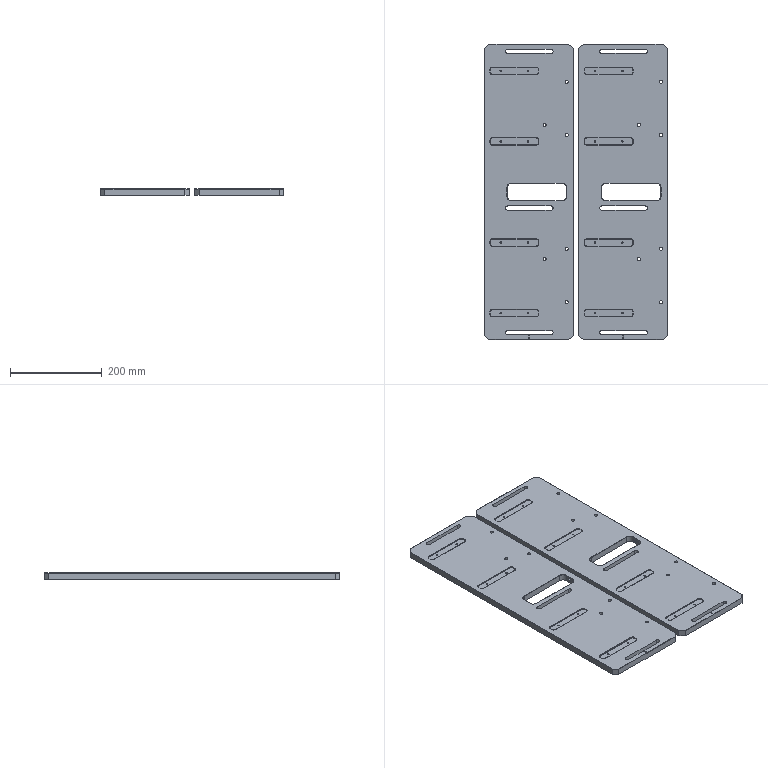NC program | NX | posted by the shop | part box 401 x 645 x 14 mm
Lines 1342 to 2472 of 5636:
N2 T06 M06
(D6  D=6. R=0. H=06 ce=0.10 di=0.10)
G00 G90 G54 X-308.9 Y102. M03 S6000
G43 H06 Z34.
M08
Z14.5
G01 Y54.5 Z14.382 F2500.
G03 X-307.5 Y53.1 Z14.377 I1.4 J0.0
X-306.1 Y54.5 Z14.371 I0.0 J1.4
G01 Y149.5 Z14.136
G03 X-307.5 Y150.9 Z14.13 I-1.4 J0.0
X-308.9 Y149.5 Z14.125 I0.0 J-1.4
G01 Y54.5 Z13.889
G03 X-307.5 Y53.1 Z13.884 I1.4 J0.0
X-306.1 Y54.5 Z13.878 I0.0 J1.4
G01 Y149.5 Z13.643
G03 X-307.5 Y150.9 Z13.637 I-1.4 J0.0
X-308.9 Y149.5 Z13.632 I0.0 J-1.4
G01 Y54.5 Z13.396
G03 X-307.5 Y53.1 Z13.391 I1.4 J0.0
X-306.1 Y54.5 Z13.385 I0.0 J1.4
G01 Y149.5 Z13.149
G03 X-307.5 Y150.9 Z13.144 I-1.4 J0.0
X-308.9 Y149.5 Z13.139 I0.0 J-1.4
G01 Y54.5 Z12.903
G03 X-307.5 Y53.1 Z12.897 I1.4 J0.0
X-306.1 Y54.5 Z12.892 I0.0 J1.4
G01 Y149.5 Z12.656
G03 X-307.5 Y150.9 Z12.651 I-1.4 J0.0
X-308.9 Y149.5 Z12.645 I0.0 J-1.4
G01 Y54.5 Z12.41
G03 X-307.5 Y53.1 Z12.404 I1.4 J0.0
X-306.1 Y54.5 Z12.399 I0.0 J1.4
G01 Y149.5 Z12.163
G03 X-307.5 Y150.9 Z12.158 I-1.4 J0.0
X-308.9 Y149.5 Z12.152 I0.0 J-1.4
G01 Y54.5 Z11.917
G03 X-307.5 Y53.1 Z11.911 I1.4 J0.0
X-306.1 Y54.5 Z11.906 I0.0 J1.4
G01 Y149.5 Z11.67
G03 X-307.5 Y150.9 Z11.665 I-1.4 J0.0
X-308.9 Y149.5 Z11.659 I0.0 J-1.4
G01 Y54.5 Z11.424
G03 X-307.5 Y53.1 Z11.418 I1.4 J0.0
X-306.1 Y54.5 Z11.413 I0.0 J1.4
G01 Y149.5 Z11.177
G03 X-307.5 Y150.9 Z11.172 I-1.4 J0.0
X-308.9 Y149.5 Z11.166 I0.0 J-1.4
G01 Y54.5 Z10.93
G03 X-307.5 Y53.1 Z10.925 I1.4 J0.0
X-306.1 Y54.5 Z10.92 I0.0 J1.4
G01 Y149.5 Z10.684
G03 X-307.5 Y150.9 Z10.678 I-1.4 J0.0
X-308.9 Y149.5 Z10.673 I0.0 J-1.4
G01 Y54.5 Z10.437
G03 X-307.5 Y53.1 Z10.432 I1.4 J0.0
X-306.1 Y54.5 Z10.426 I0.0 J1.4
G01 Y149.5 Z10.191
G03 X-307.5 Y150.9 Z10.185 I-1.4 J0.0
X-308.9 Y149.5 Z10.18 I0.0 J-1.4
G01 Y54.5 Z9.944
G03 X-307.5 Y53.1 Z9.939 I1.4 J0.0
X-306.1 Y54.5 Z9.933 I0.0 J1.4
G01 Y149.5 Z9.698
G03 X-307.5 Y150.9 Z9.692 I-1.4 J0.0
X-308.9 Y149.5 Z9.687 I0.0 J-1.4
G01 Y54.5 Z9.451
G03 X-307.5 Y53.1 Z9.446 I1.4 J0.0
X-306.1 Y54.5 Z9.44 I0.0 J1.4
G01 Y149.5 Z9.205
G03 X-307.5 Y150.9 Z9.199 I-1.4 J0.0
X-308.9 Y149.5 Z9.194 I0.0 J-1.4
G01 Y54.5 Z8.958
G03 X-307.5 Y53.1 Z8.953 I1.4 J0.0
X-306.1 Y54.5 Z8.947 I0.0 J1.4
G01 Y149.5 Z8.711
G03 X-307.5 Y150.9 Z8.706 I-1.4 J0.0
X-308.9 Y149.5 Z8.701 I0.0 J-1.4
G01 Y54.5 Z8.465
G03 X-307.5 Y53.1 Z8.459 I1.4 J0.0
X-306.1 Y54.5 Z8.454 I0.0 J1.4
G01 Y149.5 Z8.218
G03 X-307.5 Y150.9 Z8.213 I-1.4 J0.0
X-308.9 Y149.5 Z8.207 I0.0 J-1.4
G01 Y54.5 Z7.972
G03 X-307.5 Y53.1 Z7.966 I1.4 J0.0
X-306.1 Y54.5 Z7.961 I0.0 J1.4
G01 Y149.5 Z7.725
G03 X-307.5 Y150.9 Z7.72 I-1.4 J0.0
X-308.9 Y149.5 Z7.714 I0.0 J-1.4
G01 Y54.5 Z7.479
G03 X-307.5 Y53.1 Z7.473 I1.4 J0.0
X-306.1 Y54.5 Z7.468 I0.0 J1.4
G01 Y149.5 Z7.232
G03 X-307.5 Y150.9 Z7.227 I-1.4 J0.0
X-308.9 Y149.5 Z7.221 I0.0 J-1.4
G01 Y54.5 Z6.986
G03 X-307.5 Y53.1 Z6.98 I1.4 J0.0
X-306.1 Y54.5 Z6.975 I0.0 J1.4
G01 Y149.5 Z6.739
G03 X-307.5 Y150.9 Z6.734 I-1.4 J0.0
X-308.9 Y149.5 Z6.728 I0.0 J-1.4
G01 Y54.5 Z6.493
G03 X-307.5 Y53.1 Z6.487 I1.4 J0.0
X-306.1 Y54.5 Z6.482 I0.0 J1.4
G01 Y149.5 Z6.246
G03 X-307.5 Y150.9 Z6.241 I-1.4 J0.0
X-308.9 Y149.5 Z6.235 I0.0 J-1.4
G01 Y54.5 Z5.999
G03 X-307.5 Y53.1 Z5.994 I1.4 J0.0
X-306.1 Y54.5 Z5.989 I0.0 J1.4
G01 Y149.5 Z5.753
G03 X-307.5 Y150.9 Z5.747 I-1.4 J0.0
X-308.9 Y149.5 Z5.742 I0.0 J-1.4
G01 Y54.5 Z5.506
G03 X-307.5 Y53.1 Z5.501 I1.4 J0.0
X-306.1 Y54.5 Z5.495 I0.0 J1.4
G01 Y149.5 Z5.26
G03 X-307.5 Y150.9 Z5.254 I-1.4 J0.0
X-308.9 Y149.5 Z5.249 I0.0 J-1.4
G01 Y54.5 Z5.013
G03 X-307.5 Y53.1 Z5.008 I1.4 J0.0
X-306.1 Y54.5 Z5.002 I0.0 J1.4
G01 Y149.5 Z4.767
G03 X-307.5 Y150.9 Z4.761 I-1.4 J0.0
X-308.9 Y149.5 Z4.756 I0.0 J-1.4
G01 Y54.5 Z4.52
G03 X-307.5 Y53.1 Z4.515 I1.4 J0.0
X-306.1 Y54.5 Z4.509 I0.0 J1.4
G01 Y149.5 Z4.274
G03 X-307.5 Y150.9 Z4.268 I-1.4 J0.0
X-308.9 Y149.5 Z4.263 I0.0 J-1.4
G01 Y54.5 Z4.027
G03 X-307.5 Y53.1 Z4.022 I1.4 J0.0
X-306.1 Y54.5 Z4.016 I0.0 J1.4
G01 Y149.5 Z3.78
G03 X-307.5 Y150.9 Z3.775 I-1.4 J0.0
X-308.9 Y149.5 Z3.77 I0.0 J-1.4
G01 Y54.5 Z3.534
G03 X-307.5 Y53.1 Z3.528 I1.4 J0.0
X-306.1 Y54.5 Z3.523 I0.0 J1.4
G01 Y149.5 Z3.287
G03 X-307.5 Y150.9 Z3.282 I-1.4 J0.0
X-308.9 Y149.5 Z3.276 I0.0 J-1.4
G01 Y54.5 Z3.041
G03 X-307.5 Y53.1 Z3.035 I1.4 J0.0
X-306.1 Y54.5 Z3.03 I0.0 J1.4
G01 Y149.5 Z2.794
G03 X-307.5 Y150.9 Z2.789 I-1.4 J0.0
X-308.9 Y149.5 Z2.783 I0.0 J-1.4
G01 Y54.5 Z2.548
G03 X-307.5 Y53.1 Z2.542 I1.4 J0.0
X-306.1 Y54.5 Z2.537 I0.0 J1.4
G01 Y149.5 Z2.301
G03 X-307.5 Y150.9 Z2.296 I-1.4 J0.0
X-308.9 Y149.5 Z2.29 I0.0 J-1.4
G01 Y54.5 Z2.055
G03 X-307.5 Y53.1 Z2.049 I1.4 J0.0
X-306.1 Y54.5 Z2.044 I0.0 J1.4
G01 Y149.5 Z1.808
G03 X-307.5 Y150.9 Z1.803 I-1.4 J0.0
X-308.9 Y149.5 Z1.797 I0.0 J-1.4
G01 Y54.5 Z1.561
G03 X-307.5 Y53.1 Z1.556 I1.4 J0.0
X-306.1 Y54.5 Z1.551 I0.0 J1.4
G01 Y149.5 Z1.315
G03 X-307.5 Y150.9 Z1.309 I-1.4 J0.0
X-308.9 Y149.5 Z1.304 I0.0 J-1.4
G01 Y54.5 Z1.068
G03 X-307.5 Y53.1 Z1.063 I1.4 J0.0
X-306.1 Y54.5 Z1.057 I0.0 J1.4
G01 Y149.5 Z.822
G03 X-307.5 Y150.9 Z.816 I-1.4 J0.0
X-308.9 Y149.5 Z.811 I0.0 J-1.4
G01 Y54.5 Z.575
G03 X-307.5 Y53.1 Z.57 I1.4 J0.0
X-306.1 Y54.5 Z.564 I0.0 J1.4
G01 Y149.5 Z.329
G03 X-307.5 Y150.9 Z.323 I-1.4 J0.0
X-308.9 Y149.5 Z.318 I0.0 J-1.4
G01 Y102. Z.2
Y54.5
G03 X-307.5 Y53.1 I1.4 J0.0
X-306.1 Y54.5 I0.0 J1.4
G01 Y149.5
G03 X-307.5 Y150.9 I-1.4 J0.0
X-308.9 Y149.5 I0.0 J-1.4
G01 Y102.
Y101.5
Z1.2
G00 Z34.
Y-104.
Z14.5
G01 Y-151.5 Z14.382
G03 X-307.5 Y-152.9 Z14.377 I1.4 J0.0
X-306.1 Y-151.5 Z14.371 I0.0 J1.4
G01 Y-56.5 Z14.136
G03 X-307.5 Y-55.1 Z14.13 I-1.4 J0.0
X-308.9 Y-56.5 Z14.125 I0.0 J-1.4
G01 Y-151.5 Z13.889
G03 X-307.5 Y-152.9 Z13.884 I1.4 J0.0
X-306.1 Y-151.5 Z13.878 I0.0 J1.4
G01 Y-56.5 Z13.643
G03 X-307.5 Y-55.1 Z13.637 I-1.4 J0.0
X-308.9 Y-56.5 Z13.632 I0.0 J-1.4
G01 Y-151.5 Z13.396
G03 X-307.5 Y-152.9 Z13.391 I1.4 J0.0
X-306.1 Y-151.5 Z13.385 I0.0 J1.4
G01 Y-56.5 Z13.149
G03 X-307.5 Y-55.1 Z13.144 I-1.4 J0.0
X-308.9 Y-56.5 Z13.139 I0.0 J-1.4
G01 Y-151.5 Z12.903
G03 X-307.5 Y-152.9 Z12.897 I1.4 J0.0
X-306.1 Y-151.5 Z12.892 I0.0 J1.4
G01 Y-56.5 Z12.656
G03 X-307.5 Y-55.1 Z12.651 I-1.4 J0.0
X-308.9 Y-56.5 Z12.645 I0.0 J-1.4
G01 Y-151.5 Z12.41
G03 X-307.5 Y-152.9 Z12.404 I1.4 J0.0
X-306.1 Y-151.5 Z12.399 I0.0 J1.4
G01 Y-56.5 Z12.163
G03 X-307.5 Y-55.1 Z12.158 I-1.4 J0.0
X-308.9 Y-56.5 Z12.152 I0.0 J-1.4
G01 Y-151.5 Z11.917
G03 X-307.5 Y-152.9 Z11.911 I1.4 J0.0
X-306.1 Y-151.5 Z11.906 I0.0 J1.4
G01 Y-56.5 Z11.67
G03 X-307.5 Y-55.1 Z11.665 I-1.4 J0.0
X-308.9 Y-56.5 Z11.659 I0.0 J-1.4
G01 Y-151.5 Z11.424
G03 X-307.5 Y-152.9 Z11.418 I1.4 J0.0
X-306.1 Y-151.5 Z11.413 I0.0 J1.4
G01 Y-56.5 Z11.177
G03 X-307.5 Y-55.1 Z11.172 I-1.4 J0.0
X-308.9 Y-56.5 Z11.166 I0.0 J-1.4
G01 Y-151.5 Z10.93
G03 X-307.5 Y-152.9 Z10.925 I1.4 J0.0
X-306.1 Y-151.5 Z10.92 I0.0 J1.4
G01 Y-56.5 Z10.684
G03 X-307.5 Y-55.1 Z10.678 I-1.4 J0.0
X-308.9 Y-56.5 Z10.673 I0.0 J-1.4
G01 Y-151.5 Z10.437
G03 X-307.5 Y-152.9 Z10.432 I1.4 J0.0
X-306.1 Y-151.5 Z10.426 I0.0 J1.4
G01 Y-56.5 Z10.191
G03 X-307.5 Y-55.1 Z10.185 I-1.4 J0.0
X-308.9 Y-56.5 Z10.18 I0.0 J-1.4
G01 Y-151.5 Z9.944
G03 X-307.5 Y-152.9 Z9.939 I1.4 J0.0
X-306.1 Y-151.5 Z9.933 I0.0 J1.4
G01 Y-56.5 Z9.698
G03 X-307.5 Y-55.1 Z9.692 I-1.4 J0.0
X-308.9 Y-56.5 Z9.687 I0.0 J-1.4
G01 Y-151.5 Z9.451
G03 X-307.5 Y-152.9 Z9.446 I1.4 J0.0
X-306.1 Y-151.5 Z9.44 I0.0 J1.4
G01 Y-56.5 Z9.205
G03 X-307.5 Y-55.1 Z9.199 I-1.4 J0.0
X-308.9 Y-56.5 Z9.194 I0.0 J-1.4
G01 Y-151.5 Z8.958
G03 X-307.5 Y-152.9 Z8.953 I1.4 J0.0
X-306.1 Y-151.5 Z8.947 I0.0 J1.4
G01 Y-56.5 Z8.711
G03 X-307.5 Y-55.1 Z8.706 I-1.4 J0.0
X-308.9 Y-56.5 Z8.701 I0.0 J-1.4
G01 Y-151.5 Z8.465
G03 X-307.5 Y-152.9 Z8.459 I1.4 J0.0
X-306.1 Y-151.5 Z8.454 I0.0 J1.4
G01 Y-56.5 Z8.218
G03 X-307.5 Y-55.1 Z8.213 I-1.4 J0.0
X-308.9 Y-56.5 Z8.207 I0.0 J-1.4
G01 Y-151.5 Z7.972
G03 X-307.5 Y-152.9 Z7.966 I1.4 J0.0
X-306.1 Y-151.5 Z7.961 I0.0 J1.4
G01 Y-56.5 Z7.725
G03 X-307.5 Y-55.1 Z7.72 I-1.4 J0.0
X-308.9 Y-56.5 Z7.714 I0.0 J-1.4
G01 Y-151.5 Z7.479
G03 X-307.5 Y-152.9 Z7.473 I1.4 J0.0
X-306.1 Y-151.5 Z7.468 I0.0 J1.4
G01 Y-56.5 Z7.232
G03 X-307.5 Y-55.1 Z7.227 I-1.4 J0.0
X-308.9 Y-56.5 Z7.221 I0.0 J-1.4
G01 Y-151.5 Z6.986
G03 X-307.5 Y-152.9 Z6.98 I1.4 J0.0
X-306.1 Y-151.5 Z6.975 I0.0 J1.4
G01 Y-56.5 Z6.739
G03 X-307.5 Y-55.1 Z6.734 I-1.4 J0.0
X-308.9 Y-56.5 Z6.728 I0.0 J-1.4
G01 Y-151.5 Z6.493
G03 X-307.5 Y-152.9 Z6.487 I1.4 J0.0
X-306.1 Y-151.5 Z6.482 I0.0 J1.4
G01 Y-56.5 Z6.246
G03 X-307.5 Y-55.1 Z6.241 I-1.4 J0.0
X-308.9 Y-56.5 Z6.235 I0.0 J-1.4
G01 Y-151.5 Z5.999
G03 X-307.5 Y-152.9 Z5.994 I1.4 J0.0
X-306.1 Y-151.5 Z5.989 I0.0 J1.4
G01 Y-56.5 Z5.753
G03 X-307.5 Y-55.1 Z5.747 I-1.4 J0.0
X-308.9 Y-56.5 Z5.742 I0.0 J-1.4
G01 Y-151.5 Z5.506
G03 X-307.5 Y-152.9 Z5.501 I1.4 J0.0
X-306.1 Y-151.5 Z5.495 I0.0 J1.4
G01 Y-56.5 Z5.26
G03 X-307.5 Y-55.1 Z5.254 I-1.4 J0.0
X-308.9 Y-56.5 Z5.249 I0.0 J-1.4
G01 Y-151.5 Z5.013
G03 X-307.5 Y-152.9 Z5.008 I1.4 J0.0
X-306.1 Y-151.5 Z5.002 I0.0 J1.4
G01 Y-56.5 Z4.767
G03 X-307.5 Y-55.1 Z4.761 I-1.4 J0.0
X-308.9 Y-56.5 Z4.756 I0.0 J-1.4
G01 Y-151.5 Z4.52
G03 X-307.5 Y-152.9 Z4.515 I1.4 J0.0
X-306.1 Y-151.5 Z4.509 I0.0 J1.4
G01 Y-56.5 Z4.274
G03 X-307.5 Y-55.1 Z4.268 I-1.4 J0.0
X-308.9 Y-56.5 Z4.263 I0.0 J-1.4
G01 Y-151.5 Z4.027
G03 X-307.5 Y-152.9 Z4.022 I1.4 J0.0
X-306.1 Y-151.5 Z4.016 I0.0 J1.4
G01 Y-56.5 Z3.78
G03 X-307.5 Y-55.1 Z3.775 I-1.4 J0.0
X-308.9 Y-56.5 Z3.77 I0.0 J-1.4
G01 Y-151.5 Z3.534
G03 X-307.5 Y-152.9 Z3.528 I1.4 J0.0
X-306.1 Y-151.5 Z3.523 I0.0 J1.4
G01 Y-56.5 Z3.287
G03 X-307.5 Y-55.1 Z3.282 I-1.4 J0.0
X-308.9 Y-56.5 Z3.276 I0.0 J-1.4
G01 Y-151.5 Z3.041
G03 X-307.5 Y-152.9 Z3.035 I1.4 J0.0
X-306.1 Y-151.5 Z3.03 I0.0 J1.4
G01 Y-56.5 Z2.794
G03 X-307.5 Y-55.1 Z2.789 I-1.4 J0.0
X-308.9 Y-56.5 Z2.783 I0.0 J-1.4
G01 Y-151.5 Z2.548
G03 X-307.5 Y-152.9 Z2.542 I1.4 J0.0
X-306.1 Y-151.5 Z2.537 I0.0 J1.4
G01 Y-56.5 Z2.301
G03 X-307.5 Y-55.1 Z2.296 I-1.4 J0.0
X-308.9 Y-56.5 Z2.29 I0.0 J-1.4
G01 Y-151.5 Z2.055
G03 X-307.5 Y-152.9 Z2.049 I1.4 J0.0
X-306.1 Y-151.5 Z2.044 I0.0 J1.4
G01 Y-56.5 Z1.808
G03 X-307.5 Y-55.1 Z1.803 I-1.4 J0.0
X-308.9 Y-56.5 Z1.797 I0.0 J-1.4
G01 Y-151.5 Z1.561
G03 X-307.5 Y-152.9 Z1.556 I1.4 J0.0
X-306.1 Y-151.5 Z1.551 I0.0 J1.4
G01 Y-56.5 Z1.315
G03 X-307.5 Y-55.1 Z1.309 I-1.4 J0.0
X-308.9 Y-56.5 Z1.304 I0.0 J-1.4
G01 Y-151.5 Z1.068
G03 X-307.5 Y-152.9 Z1.063 I1.4 J0.0
X-306.1 Y-151.5 Z1.057 I0.0 J1.4
G01 Y-56.5 Z.822
G03 X-307.5 Y-55.1 Z.816 I-1.4 J0.0
X-308.9 Y-56.5 Z.811 I0.0 J-1.4
G01 Y-151.5 Z.575
G03 X-307.5 Y-152.9 Z.57 I1.4 J0.0
X-306.1 Y-151.5 Z.564 I0.0 J1.4
G01 Y-56.5 Z.329
G03 X-307.5 Y-55.1 Z.323 I-1.4 J0.0
X-308.9 Y-56.5 Z.318 I0.0 J-1.4
G01 Y-104. Z.2
Y-151.5
G03 X-307.5 Y-152.9 I1.4 J0.0
X-306.1 Y-151.5 I0.0 J1.4
G01 Y-56.5
G03 X-307.5 Y-55.1 I-1.4 J0.0
X-308.9 Y-56.5 I0.0 J-1.4
G01 Y-104.
Y-104.5
Z1.2
G00 Z34.
X-36.4 Y-104.
Z14.5
G01 Y-151.5 Z14.382
G03 X-35. Y-152.9 Z14.377 I1.4 J0.0
X-33.6 Y-151.5 Z14.371 I0.0 J1.4
G01 Y-56.5 Z14.136
G03 X-35. Y-55.1 Z14.13 I-1.4 J0.0
X-36.4 Y-56.5 Z14.125 I0.0 J-1.4
G01 Y-151.5 Z13.889
G03 X-35. Y-152.9 Z13.884 I1.4 J0.0
X-33.6 Y-151.5 Z13.878 I0.0 J1.4
G01 Y-56.5 Z13.643
G03 X-35. Y-55.1 Z13.637 I-1.4 J0.0
X-36.4 Y-56.5 Z13.632 I0.0 J-1.4
G01 Y-151.5 Z13.396
G03 X-35. Y-152.9 Z13.391 I1.4 J0.0
X-33.6 Y-151.5 Z13.385 I0.0 J1.4
G01 Y-56.5 Z13.149
G03 X-35. Y-55.1 Z13.144 I-1.4 J0.0
X-36.4 Y-56.5 Z13.139 I0.0 J-1.4
G01 Y-151.5 Z12.903
G03 X-35. Y-152.9 Z12.897 I1.4 J0.0
X-33.6 Y-151.5 Z12.892 I0.0 J1.4
G01 Y-56.5 Z12.656
G03 X-35. Y-55.1 Z12.651 I-1.4 J0.0
X-36.4 Y-56.5 Z12.645 I0.0 J-1.4
G01 Y-151.5 Z12.41
G03 X-35. Y-152.9 Z12.404 I1.4 J0.0
X-33.6 Y-151.5 Z12.399 I0.0 J1.4
G01 Y-56.5 Z12.163
G03 X-35. Y-55.1 Z12.158 I-1.4 J0.0
X-36.4 Y-56.5 Z12.152 I0.0 J-1.4
G01 Y-151.5 Z11.917
G03 X-35. Y-152.9 Z11.911 I1.4 J0.0
X-33.6 Y-151.5 Z11.906 I0.0 J1.4
G01 Y-56.5 Z11.67
G03 X-35. Y-55.1 Z11.665 I-1.4 J0.0
X-36.4 Y-56.5 Z11.659 I0.0 J-1.4
G01 Y-151.5 Z11.424
G03 X-35. Y-152.9 Z11.418 I1.4 J0.0
X-33.6 Y-151.5 Z11.413 I0.0 J1.4
G01 Y-56.5 Z11.177
G03 X-35. Y-55.1 Z11.172 I-1.4 J0.0
X-36.4 Y-56.5 Z11.166 I0.0 J-1.4
G01 Y-151.5 Z10.93
G03 X-35. Y-152.9 Z10.925 I1.4 J0.0
X-33.6 Y-151.5 Z10.92 I0.0 J1.4
G01 Y-56.5 Z10.684
G03 X-35. Y-55.1 Z10.678 I-1.4 J0.0
X-36.4 Y-56.5 Z10.673 I0.0 J-1.4
G01 Y-151.5 Z10.437
G03 X-35. Y-152.9 Z10.432 I1.4 J0.0
X-33.6 Y-151.5 Z10.426 I0.0 J1.4
G01 Y-56.5 Z10.191
G03 X-35. Y-55.1 Z10.185 I-1.4 J0.0
X-36.4 Y-56.5 Z10.18 I0.0 J-1.4
G01 Y-151.5 Z9.944
G03 X-35. Y-152.9 Z9.939 I1.4 J0.0
X-33.6 Y-151.5 Z9.933 I0.0 J1.4
G01 Y-56.5 Z9.698
G03 X-35. Y-55.1 Z9.692 I-1.4 J0.0
X-36.4 Y-56.5 Z9.687 I0.0 J-1.4
G01 Y-151.5 Z9.451
G03 X-35. Y-152.9 Z9.446 I1.4 J0.0
X-33.6 Y-151.5 Z9.44 I0.0 J1.4
G01 Y-56.5 Z9.205
G03 X-35. Y-55.1 Z9.199 I-1.4 J0.0
X-36.4 Y-56.5 Z9.194 I0.0 J-1.4
G01 Y-151.5 Z8.958
G03 X-35. Y-152.9 Z8.953 I1.4 J0.0
X-33.6 Y-151.5 Z8.947 I0.0 J1.4
G01 Y-56.5 Z8.711
G03 X-35. Y-55.1 Z8.706 I-1.4 J0.0
X-36.4 Y-56.5 Z8.701 I0.0 J-1.4
G01 Y-151.5 Z8.465
G03 X-35. Y-152.9 Z8.459 I1.4 J0.0
X-33.6 Y-151.5 Z8.454 I0.0 J1.4
G01 Y-56.5 Z8.218
G03 X-35. Y-55.1 Z8.213 I-1.4 J0.0
X-36.4 Y-56.5 Z8.207 I0.0 J-1.4
G01 Y-151.5 Z7.972
G03 X-35. Y-152.9 Z7.966 I1.4 J0.0
X-33.6 Y-151.5 Z7.961 I0.0 J1.4
G01 Y-56.5 Z7.725
G03 X-35. Y-55.1 Z7.72 I-1.4 J0.0
X-36.4 Y-56.5 Z7.714 I0.0 J-1.4
G01 Y-151.5 Z7.479
G03 X-35. Y-152.9 Z7.473 I1.4 J0.0
X-33.6 Y-151.5 Z7.468 I0.0 J1.4
G01 Y-56.5 Z7.232
G03 X-35. Y-55.1 Z7.227 I-1.4 J0.0
X-36.4 Y-56.5 Z7.221 I0.0 J-1.4
G01 Y-151.5 Z6.986
G03 X-35. Y-152.9 Z6.98 I1.4 J0.0
X-33.6 Y-151.5 Z6.975 I0.0 J1.4
G01 Y-56.5 Z6.739
G03 X-35. Y-55.1 Z6.734 I-1.4 J0.0
X-36.4 Y-56.5 Z6.728 I0.0 J-1.4
G01 Y-151.5 Z6.493
G03 X-35. Y-152.9 Z6.487 I1.4 J0.0
X-33.6 Y-151.5 Z6.482 I0.0 J1.4
G01 Y-56.5 Z6.246
G03 X-35. Y-55.1 Z6.241 I-1.4 J0.0
X-36.4 Y-56.5 Z6.235 I0.0 J-1.4
G01 Y-151.5 Z5.999
G03 X-35. Y-152.9 Z5.994 I1.4 J0.0
X-33.6 Y-151.5 Z5.989 I0.0 J1.4
G01 Y-56.5 Z5.753
G03 X-35. Y-55.1 Z5.747 I-1.4 J0.0
X-36.4 Y-56.5 Z5.742 I0.0 J-1.4
G01 Y-151.5 Z5.506
G03 X-35. Y-152.9 Z5.501 I1.4 J0.0
X-33.6 Y-151.5 Z5.495 I0.0 J1.4
G01 Y-56.5 Z5.26
G03 X-35. Y-55.1 Z5.254 I-1.4 J0.0
X-36.4 Y-56.5 Z5.249 I0.0 J-1.4
G01 Y-151.5 Z5.013
G03 X-35. Y-152.9 Z5.008 I1.4 J0.0
X-33.6 Y-151.5 Z5.002 I0.0 J1.4
G01 Y-56.5 Z4.767
G03 X-35. Y-55.1 Z4.761 I-1.4 J0.0
X-36.4 Y-56.5 Z4.756 I0.0 J-1.4
G01 Y-151.5 Z4.52
G03 X-35. Y-152.9 Z4.515 I1.4 J0.0
X-33.6 Y-151.5 Z4.509 I0.0 J1.4
G01 Y-56.5 Z4.274
G03 X-35. Y-55.1 Z4.268 I-1.4 J0.0
X-36.4 Y-56.5 Z4.263 I0.0 J-1.4
G01 Y-151.5 Z4.027
G03 X-35. Y-152.9 Z4.022 I1.4 J0.0
X-33.6 Y-151.5 Z4.016 I0.0 J1.4
G01 Y-56.5 Z3.78
G03 X-35. Y-55.1 Z3.775 I-1.4 J0.0
X-36.4 Y-56.5 Z3.77 I0.0 J-1.4
G01 Y-151.5 Z3.534
G03 X-35. Y-152.9 Z3.528 I1.4 J0.0
X-33.6 Y-151.5 Z3.523 I0.0 J1.4
G01 Y-56.5 Z3.287
G03 X-35. Y-55.1 Z3.282 I-1.4 J0.0
X-36.4 Y-56.5 Z3.276 I0.0 J-1.4
G01 Y-151.5 Z3.041
G03 X-35. Y-152.9 Z3.035 I1.4 J0.0
X-33.6 Y-151.5 Z3.03 I0.0 J1.4
G01 Y-56.5 Z2.794
G03 X-35. Y-55.1 Z2.789 I-1.4 J0.0
X-36.4 Y-56.5 Z2.783 I0.0 J-1.4
G01 Y-151.5 Z2.548
G03 X-35. Y-152.9 Z2.542 I1.4 J0.0
X-33.6 Y-151.5 Z2.537 I0.0 J1.4
G01 Y-56.5 Z2.301
G03 X-35. Y-55.1 Z2.296 I-1.4 J0.0
X-36.4 Y-56.5 Z2.29 I0.0 J-1.4
G01 Y-151.5 Z2.055
G03 X-35. Y-152.9 Z2.049 I1.4 J0.0
X-33.6 Y-151.5 Z2.044 I0.0 J1.4
G01 Y-56.5 Z1.808
G03 X-35. Y-55.1 Z1.803 I-1.4 J0.0
X-36.4 Y-56.5 Z1.797 I0.0 J-1.4
G01 Y-151.5 Z1.561
G03 X-35. Y-152.9 Z1.556 I1.4 J0.0
X-33.6 Y-151.5 Z1.551 I0.0 J1.4
G01 Y-56.5 Z1.315
G03 X-35. Y-55.1 Z1.309 I-1.4 J0.0
X-36.4 Y-56.5 Z1.304 I0.0 J-1.4
G01 Y-151.5 Z1.068
G03 X-35. Y-152.9 Z1.063 I1.4 J0.0
X-33.6 Y-151.5 Z1.057 I0.0 J1.4
G01 Y-56.5 Z.822
G03 X-35. Y-55.1 Z.816 I-1.4 J0.0
X-36.4 Y-56.5 Z.811 I0.0 J-1.4
G01 Y-151.5 Z.575
G03 X-35. Y-152.9 Z.57 I1.4 J0.0
X-33.6 Y-151.5 Z.564 I0.0 J1.4
G01 Y-56.5 Z.329
G03 X-35. Y-55.1 Z.323 I-1.4 J0.0
X-36.4 Y-56.5 Z.318 I0.0 J-1.4
G01 Y-104. Z.2
Y-151.5
G03 X-35. Y-152.9 I1.4 J0.0
X-33.6 Y-151.5 I0.0 J1.4
G01 Y-56.5
G03 X-35. Y-55.1 I-1.4 J0.0
X-36.4 Y-56.5 I0.0 J-1.4
G01 Y-104.
Y-104.5
Z1.2
G00 Z34.
Y102.
Z14.5
G01 Y54.5 Z14.382
G03 X-35. Y53.1 Z14.377 I1.4 J0.0
X-33.6 Y54.5 Z14.371 I0.0 J1.4
G01 Y149.5 Z14.136
G03 X-35. Y150.9 Z14.13 I-1.4 J0.0
X-36.4 Y149.5 Z14.125 I0.0 J-1.4
G01 Y54.5 Z13.889
G03 X-35. Y53.1 Z13.884 I1.4 J0.0
X-33.6 Y54.5 Z13.878 I0.0 J1.4
G01 Y149.5 Z13.643
G03 X-35. Y150.9 Z13.637 I-1.4 J0.0
X-36.4 Y149.5 Z13.632 I0.0 J-1.4
G01 Y54.5 Z13.396
G03 X-35. Y53.1 Z13.391 I1.4 J0.0
X-33.6 Y54.5 Z13.385 I0.0 J1.4
G01 Y149.5 Z13.149
G03 X-35. Y150.9 Z13.144 I-1.4 J0.0
X-36.4 Y149.5 Z13.139 I0.0 J-1.4
G01 Y54.5 Z12.903
G03 X-35. Y53.1 Z12.897 I1.4 J0.0
X-33.6 Y54.5 Z12.892 I0.0 J1.4
G01 Y149.5 Z12.656
G03 X-35. Y150.9 Z12.651 I-1.4 J0.0
X-36.4 Y149.5 Z12.645 I0.0 J-1.4
G01 Y54.5 Z12.41
G03 X-35. Y53.1 Z12.404 I1.4 J0.0
X-33.6 Y54.5 Z12.399 I0.0 J1.4
G01 Y149.5 Z12.163
G03 X-35. Y150.9 Z12.158 I-1.4 J0.0
X-36.4 Y149.5 Z12.152 I0.0 J-1.4
G01 Y54.5 Z11.917
G03 X-35. Y53.1 Z11.911 I1.4 J0.0
X-33.6 Y54.5 Z11.906 I0.0 J1.4
G01 Y149.5 Z11.67
G03 X-35. Y150.9 Z11.665 I-1.4 J0.0
X-36.4 Y149.5 Z11.659 I0.0 J-1.4
G01 Y54.5 Z11.424
G03 X-35. Y53.1 Z11.418 I1.4 J0.0
X-33.6 Y54.5 Z11.413 I0.0 J1.4
G01 Y149.5 Z11.177
G03 X-35. Y150.9 Z11.172 I-1.4 J0.0
X-36.4 Y149.5 Z11.166 I0.0 J-1.4
G01 Y54.5 Z10.93
G03 X-35. Y53.1 Z10.925 I1.4 J0.0
X-33.6 Y54.5 Z10.92 I0.0 J1.4
G01 Y149.5 Z10.684
G03 X-35. Y150.9 Z10.678 I-1.4 J0.0
X-36.4 Y149.5 Z10.673 I0.0 J-1.4
G01 Y54.5 Z10.437
G03 X-35. Y53.1 Z10.432 I1.4 J0.0
X-33.6 Y54.5 Z10.426 I0.0 J1.4
G01 Y149.5 Z10.191
G03 X-35. Y150.9 Z10.185 I-1.4 J0.0
X-36.4 Y149.5 Z10.18 I0.0 J-1.4
G01 Y54.5 Z9.944
G03 X-35. Y53.1 Z9.939 I1.4 J0.0
X-33.6 Y54.5 Z9.933 I0.0 J1.4
G01 Y149.5 Z9.698
G03 X-35. Y150.9 Z9.692 I-1.4 J0.0
X-36.4 Y149.5 Z9.687 I0.0 J-1.4
G01 Y54.5 Z9.451
G03 X-35. Y53.1 Z9.446 I1.4 J0.0
X-33.6 Y54.5 Z9.44 I0.0 J1.4
G01 Y149.5 Z9.205
G03 X-35. Y150.9 Z9.199 I-1.4 J0.0
X-36.4 Y149.5 Z9.194 I0.0 J-1.4
G01 Y54.5 Z8.958
G03 X-35. Y53.1 Z8.953 I1.4 J0.0
X-33.6 Y54.5 Z8.947 I0.0 J1.4
G01 Y149.5 Z8.711
G03 X-35. Y150.9 Z8.706 I-1.4 J0.0
X-36.4 Y149.5 Z8.701 I0.0 J-1.4
G01 Y54.5 Z8.465
G03 X-35. Y53.1 Z8.459 I1.4 J0.0
X-33.6 Y54.5 Z8.454 I0.0 J1.4
G01 Y149.5 Z8.218
G03 X-35. Y150.9 Z8.213 I-1.4 J0.0
X-36.4 Y149.5 Z8.207 I0.0 J-1.4
G01 Y54.5 Z7.972
G03 X-35. Y53.1 Z7.966 I1.4 J0.0
X-33.6 Y54.5 Z7.961 I0.0 J1.4
G01 Y149.5 Z7.725
G03 X-35. Y150.9 Z7.72 I-1.4 J0.0
X-36.4 Y149.5 Z7.714 I0.0 J-1.4
G01 Y54.5 Z7.479
G03 X-35. Y53.1 Z7.473 I1.4 J0.0
X-33.6 Y54.5 Z7.468 I0.0 J1.4
G01 Y149.5 Z7.232
G03 X-35. Y150.9 Z7.227 I-1.4 J0.0
X-36.4 Y149.5 Z7.221 I0.0 J-1.4
G01 Y54.5 Z6.986
G03 X-35. Y53.1 Z6.98 I1.4 J0.0
X-33.6 Y54.5 Z6.975 I0.0 J1.4
G01 Y149.5 Z6.739
G03 X-35. Y150.9 Z6.734 I-1.4 J0.0
X-36.4 Y149.5 Z6.728 I0.0 J-1.4
G01 Y54.5 Z6.493
G03 X-35. Y53.1 Z6.487 I1.4 J0.0
X-33.6 Y54.5 Z6.482 I0.0 J1.4
G01 Y149.5 Z6.246
G03 X-35. Y150.9 Z6.241 I-1.4 J0.0
X-36.4 Y149.5 Z6.235 I0.0 J-1.4
G01 Y54.5 Z5.999
G03 X-35. Y53.1 Z5.994 I1.4 J0.0
X-33.6 Y54.5 Z5.989 I0.0 J1.4
G01 Y149.5 Z5.753
G03 X-35. Y150.9 Z5.747 I-1.4 J0.0
X-36.4 Y149.5 Z5.742 I0.0 J-1.4
G01 Y54.5 Z5.506
G03 X-35. Y53.1 Z5.501 I1.4 J0.0
X-33.6 Y54.5 Z5.495 I0.0 J1.4
G01 Y149.5 Z5.26
G03 X-35. Y150.9 Z5.254 I-1.4 J0.0
X-36.4 Y149.5 Z5.249 I0.0 J-1.4
G01 Y54.5 Z5.013
G03 X-35. Y53.1 Z5.008 I1.4 J0.0
X-33.6 Y54.5 Z5.002 I0.0 J1.4
G01 Y149.5 Z4.767
G03 X-35. Y150.9 Z4.761 I-1.4 J0.0
X-36.4 Y149.5 Z4.756 I0.0 J-1.4
G01 Y54.5 Z4.52
G03 X-35. Y53.1 Z4.515 I1.4 J0.0
X-33.6 Y54.5 Z4.509 I0.0 J1.4
G01 Y149.5 Z4.274
G03 X-35. Y150.9 Z4.268 I-1.4 J0.0
X-36.4 Y149.5 Z4.263 I0.0 J-1.4
G01 Y54.5 Z4.027
G03 X-35. Y53.1 Z4.022 I1.4 J0.0
X-33.6 Y54.5 Z4.016 I0.0 J1.4
G01 Y149.5 Z3.78
G03 X-35. Y150.9 Z3.775 I-1.4 J0.0
X-36.4 Y149.5 Z3.77 I0.0 J-1.4
G01 Y54.5 Z3.534
G03 X-35. Y53.1 Z3.528 I1.4 J0.0
X-33.6 Y54.5 Z3.523 I0.0 J1.4
G01 Y149.5 Z3.287
G03 X-35. Y150.9 Z3.282 I-1.4 J0.0
X-36.4 Y149.5 Z3.276 I0.0 J-1.4
G01 Y54.5 Z3.041
G03 X-35. Y53.1 Z3.035 I1.4 J0.0
X-33.6 Y54.5 Z3.03 I0.0 J1.4
G01 Y149.5 Z2.794
G03 X-35. Y150.9 Z2.789 I-1.4 J0.0
X-36.4 Y149.5 Z2.783 I0.0 J-1.4
G01 Y54.5 Z2.548
G03 X-35. Y53.1 Z2.542 I1.4 J0.0
X-33.6 Y54.5 Z2.537 I0.0 J1.4
G01 Y149.5 Z2.301
G03 X-35. Y150.9 Z2.296 I-1.4 J0.0
X-36.4 Y149.5 Z2.29 I0.0 J-1.4
G01 Y54.5 Z2.055
G03 X-35. Y53.1 Z2.049 I1.4 J0.0
X-33.6 Y54.5 Z2.044 I0.0 J1.4
G01 Y149.5 Z1.808
G03 X-35. Y150.9 Z1.803 I-1.4 J0.0
X-36.4 Y149.5 Z1.797 I0.0 J-1.4
G01 Y54.5 Z1.561
G03 X-35. Y53.1 Z1.556 I1.4 J0.0
X-33.6 Y54.5 Z1.551 I0.0 J1.4
G01 Y149.5 Z1.315
G03 X-35. Y150.9 Z1.309 I-1.4 J0.0
X-36.4 Y149.5 Z1.304 I0.0 J-1.4
G01 Y54.5 Z1.068
G03 X-35. Y53.1 Z1.063 I1.4 J0.0
X-33.6 Y54.5 Z1.057 I0.0 J1.4
G01 Y149.5 Z.822
G03 X-35. Y150.9 Z.816 I-1.4 J0.0
X-36.4 Y149.5 Z.811 I0.0 J-1.4
G01 Y54.5 Z.575
G03 X-35. Y53.1 Z.57 I1.4 J0.0
X-33.6 Y54.5 Z.564 I0.0 J1.4
G01 Y149.5 Z.329
G03 X-35. Y150.9 Z.323 I-1.4 J0.0
X-36.4 Y149.5 Z.318 I0.0 J-1.4
G01 Y102. Z.2
Y54.5
G03 X-35. Y53.1 I1.4 J0.0
X-33.6 Y54.5 I0.0 J1.4
G01 Y149.5
G03 X-35. Y150.9 I-1.4 J0.0
X-36.4 Y149.5 I0.0 J-1.4
G01 Y102.
Y101.5
Z1.2
G00 Z34.
X308.9 Y102.
Z14.5
G01 Y149.5 Z14.382
G03 X307.5 Y150.9 Z14.377 I-1.4 J0.0
X306.1 Y149.5 Z14.371 I0.0 J-1.4
G01 Y54.5 Z14.136
G03 X307.5 Y53.1 Z14.13 I1.4 J0.0
X308.9 Y54.5 Z14.125 I0.0 J1.4
G01 Y149.5 Z13.889
G03 X307.5 Y150.9 Z13.884 I-1.4 J0.0
X306.1 Y149.5 Z13.878 I0.0 J-1.4
G01 Y54.5 Z13.643
G03 X307.5 Y53.1 Z13.637 I1.4 J0.0
X308.9 Y54.5 Z13.632 I0.0 J1.4
G01 Y149.5 Z13.396
G03 X307.5 Y150.9 Z13.391 I-1.4 J0.0
X306.1 Y149.5 Z13.385 I0.0 J-1.4
G01 Y54.5 Z13.149
G03 X307.5 Y53.1 Z13.144 I1.4 J0.0
X308.9 Y54.5 Z13.139 I0.0 J1.4
G01 Y149.5 Z12.903
G03 X307.5 Y150.9 Z12.897 I-1.4 J0.0
X306.1 Y149.5 Z12.892 I0.0 J-1.4
G01 Y54.5 Z12.656
G03 X307.5 Y53.1 Z12.651 I1.4 J0.0
X308.9 Y54.5 Z12.645 I0.0 J1.4
G01 Y149.5 Z12.41
G03 X307.5 Y150.9 Z12.404 I-1.4 J0.0
X306.1 Y149.5 Z12.399 I0.0 J-1.4
G01 Y54.5 Z12.163
G03 X307.5 Y53.1 Z12.158 I1.4 J0.0
X308.9 Y54.5 Z12.152 I0.0 J1.4
G01 Y149.5 Z11.917
G03 X307.5 Y150.9 Z11.911 I-1.4 J0.0
X306.1 Y149.5 Z11.906 I0.0 J-1.4
G01 Y54.5 Z11.67
G03 X307.5 Y53.1 Z11.665 I1.4 J0.0
X308.9 Y54.5 Z11.659 I0.0 J1.4
G01 Y149.5 Z11.424
G03 X307.5 Y150.9 Z11.418 I-1.4 J0.0
X306.1 Y149.5 Z11.413 I0.0 J-1.4
G01 Y54.5 Z11.177
G03 X307.5 Y53.1 Z11.172 I1.4 J0.0
X308.9 Y54.5 Z11.166 I0.0 J1.4
G01 Y149.5 Z10.93
G03 X307.5 Y150.9 Z10.925 I-1.4 J0.0
X306.1 Y149.5 Z10.92 I0.0 J-1.4
G01 Y54.5 Z10.684
G03 X307.5 Y53.1 Z10.678 I1.4 J0.0
X308.9 Y54.5 Z10.673 I0.0 J1.4
G01 Y149.5 Z10.437
G03 X307.5 Y150.9 Z10.432 I-1.4 J0.0
X306.1 Y149.5 Z10.426 I0.0 J-1.4
G01 Y54.5 Z10.191
G03 X307.5 Y53.1 Z10.185 I1.4 J0.0
X308.9 Y54.5 Z10.18 I0.0 J1.4
G01 Y149.5 Z9.944
G03 X307.5 Y150.9 Z9.939 I-1.4 J0.0
X306.1 Y149.5 Z9.933 I0.0 J-1.4
G01 Y54.5 Z9.698
G03 X307.5 Y53.1 Z9.692 I1.4 J0.0
X308.9 Y54.5 Z9.687 I0.0 J1.4
G01 Y149.5 Z9.451
G03 X307.5 Y150.9 Z9.446 I-1.4 J0.0
X306.1 Y149.5 Z9.44 I0.0 J-1.4
G01 Y54.5 Z9.205
G03 X307.5 Y53.1 Z9.199 I1.4 J0.0
X308.9 Y54.5 Z9.194 I0.0 J1.4
G01 Y149.5 Z8.958
G03 X307.5 Y150.9 Z8.953 I-1.4 J0.0
X306.1 Y149.5 Z8.947 I0.0 J-1.4
G01 Y54.5 Z8.711
G03 X307.5 Y53.1 Z8.706 I1.4 J0.0
X308.9 Y54.5 Z8.701 I0.0 J1.4
G01 Y149.5 Z8.465
G03 X307.5 Y150.9 Z8.459 I-1.4 J0.0
X306.1 Y149.5 Z8.454 I0.0 J-1.4
G01 Y54.5 Z8.218
G03 X307.5 Y53.1 Z8.213 I1.4 J0.0
X308.9 Y54.5 Z8.207 I0.0 J1.4
G01 Y149.5 Z7.972
G03 X307.5 Y150.9 Z7.966 I-1.4 J0.0
X306.1 Y149.5 Z7.961 I0.0 J-1.4
G01 Y54.5 Z7.725
G03 X307.5 Y53.1 Z7.72 I1.4 J0.0
X308.9 Y54.5 Z7.714 I0.0 J1.4
G01 Y149.5 Z7.479
G03 X307.5 Y150.9 Z7.473 I-1.4 J0.0
X306.1 Y149.5 Z7.468 I0.0 J-1.4
G01 Y54.5 Z7.232
G03 X307.5 Y53.1 Z7.227 I1.4 J0.0
X308.9 Y54.5 Z7.221 I0.0 J1.4
G01 Y149.5 Z6.986
G03 X307.5 Y150.9 Z6.98 I-1.4 J0.0
X306.1 Y149.5 Z6.975 I0.0 J-1.4
G01 Y54.5 Z6.739
G03 X307.5 Y53.1 Z6.734 I1.4 J0.0
X308.9 Y54.5 Z6.728 I0.0 J1.4
G01 Y149.5 Z6.493
G03 X307.5 Y150.9 Z6.487 I-1.4 J0.0
X306.1 Y149.5 Z6.482 I0.0 J-1.4
G01 Y54.5 Z6.246
G03 X307.5 Y53.1 Z6.241 I1.4 J0.0
X308.9 Y54.5 Z6.235 I0.0 J1.4
G01 Y149.5 Z5.999
G03 X307.5 Y150.9 Z5.994 I-1.4 J0.0
X306.1 Y149.5 Z5.989 I0.0 J-1.4
G01 Y54.5 Z5.753
G03 X307.5 Y53.1 Z5.747 I1.4 J0.0
X308.9 Y54.5 Z5.742 I0.0 J1.4
G01 Y149.5 Z5.506
G03 X307.5 Y150.9 Z5.501 I-1.4 J0.0
X306.1 Y149.5 Z5.495 I0.0 J-1.4
G01 Y54.5 Z5.26
G03 X307.5 Y53.1 Z5.254 I1.4 J0.0
X308.9 Y54.5 Z5.249 I0.0 J1.4
G01 Y149.5 Z5.013
G03 X307.5 Y150.9 Z5.008 I-1.4 J0.0
X306.1 Y149.5 Z5.002 I0.0 J-1.4
G01 Y54.5 Z4.767
G03 X307.5 Y53.1 Z4.761 I1.4 J0.0
X308.9 Y54.5 Z4.756 I0.0 J1.4
G01 Y149.5 Z4.52
G03 X307.5 Y150.9 Z4.515 I-1.4 J0.0
X306.1 Y149.5 Z4.509 I0.0 J-1.4
G01 Y54.5 Z4.274
G03 X307.5 Y53.1 Z4.268 I1.4 J0.0
X308.9 Y54.5 Z4.263 I0.0 J1.4
G01 Y149.5 Z4.027
G03 X307.5 Y150.9 Z4.022 I-1.4 J0.0
X306.1 Y149.5 Z4.016 I0.0 J-1.4
G01 Y54.5 Z3.78
G03 X307.5 Y53.1 Z3.775 I1.4 J0.0
X308.9 Y54.5 Z3.77 I0.0 J1.4
G01 Y149.5 Z3.534
G03 X307.5 Y150.9 Z3.528 I-1.4 J0.0
X306.1 Y149.5 Z3.523 I0.0 J-1.4
G01 Y54.5 Z3.287
G03 X307.5 Y53.1 Z3.282 I1.4 J0.0
X308.9 Y54.5 Z3.276 I0.0 J1.4
G01 Y149.5 Z3.041
G03 X307.5 Y150.9 Z3.035 I-1.4 J0.0
X306.1 Y149.5 Z3.03 I0.0 J-1.4
G01 Y54.5 Z2.794
G03 X307.5 Y53.1 Z2.789 I1.4 J0.0
X308.9 Y54.5 Z2.783 I0.0 J1.4
G01 Y149.5 Z2.548
G03 X307.5 Y150.9 Z2.542 I-1.4 J0.0
X306.1 Y149.5 Z2.537 I0.0 J-1.4
G01 Y54.5 Z2.301
G03 X307.5 Y53.1 Z2.296 I1.4 J0.0
X308.9 Y54.5 Z2.29 I0.0 J1.4
G01 Y149.5 Z2.055
G03 X307.5 Y150.9 Z2.049 I-1.4 J0.0
X306.1 Y149.5 Z2.044 I0.0 J-1.4
G01 Y54.5 Z1.808
G03 X307.5 Y53.1 Z1.803 I1.4 J0.0
X308.9 Y54.5 Z1.797 I0.0 J1.4
G01 Y149.5 Z1.561
G03 X307.5 Y150.9 Z1.556 I-1.4 J0.0
X306.1 Y149.5 Z1.551 I0.0 J-1.4
G01 Y54.5 Z1.315
G03 X307.5 Y53.1 Z1.309 I1.4 J0.0
X308.9 Y54.5 Z1.304 I0.0 J1.4
G01 Y149.5 Z1.068
G03 X307.5 Y150.9 Z1.063 I-1.4 J0.0
X306.1 Y149.5 Z1.057 I0.0 J-1.4
G01 Y54.5 Z.822
G03 X307.5 Y53.1 Z.816 I1.4 J0.0
X308.9 Y54.5 Z.811 I0.0 J1.4
G01 Y149.5 Z.575
G03 X307.5 Y150.9 Z.57 I-1.4 J0.0
X306.1 Y149.5 Z.564 I0.0 J-1.4
G01 Y54.5 Z.329
G03 X307.5 Y53.1 Z.323 I1.4 J0.0
X308.9 Y54.5 Z.318 I0.0 J1.4
G01 Y102. Z.2
Y149.5
G03 X307.5 Y150.9 I-1.4 J0.0
X306.1 Y149.5 I0.0 J-1.4
G01 Y54.5
G03 X307.5 Y53.1 I1.4 J0.0
X308.9 Y54.5 I0.0 J1.4
G01 Y102.
Y102.5
Z1.2
G00 Z34.
Y-104.
Z14.5
G01 Y-56.5 Z14.382
G03 X307.5 Y-55.1 Z14.377 I-1.4 J0.0
X306.1 Y-56.5 Z14.371 I0.0 J-1.4
G01 Y-151.5 Z14.136
G03 X307.5 Y-152.9 Z14.13 I1.4 J0.0
X308.9 Y-151.5 Z14.125 I0.0 J1.4
G01 Y-56.5 Z13.889
G03 X307.5 Y-55.1 Z13.884 I-1.4 J0.0
X306.1 Y-56.5 Z13.878 I0.0 J-1.4
G01 Y-151.5 Z13.643
G03 X307.5 Y-152.9 Z13.637 I1.4 J0.0
X308.9 Y-151.5 Z13.632 I0.0 J1.4
G01 Y-56.5 Z13.396
G03 X307.5 Y-55.1 Z13.391 I-1.4 J0.0
X306.1 Y-56.5 Z13.385 I0.0 J-1.4
G01 Y-151.5 Z13.149
G03 X307.5 Y-152.9 Z13.144 I1.4 J0.0
X308.9 Y-151.5 Z13.139 I0.0 J1.4
G01 Y-56.5 Z12.903
G03 X307.5 Y-55.1 Z12.897 I-1.4 J0.0
X306.1 Y-56.5 Z12.892 I0.0 J-1.4
G01 Y-151.5 Z12.656
G03 X307.5 Y-152.9 Z12.651 I1.4 J0.0
X308.9 Y-151.5 Z12.645 I0.0 J1.4
G01 Y-56.5 Z12.41
G03 X307.5 Y-55.1 Z12.404 I-1.4 J0.0
X306.1 Y-56.5 Z12.399 I0.0 J-1.4
G01 Y-151.5 Z12.163
G03 X307.5 Y-152.9 Z12.158 I1.4 J0.0
X308.9 Y-151.5 Z12.152 I0.0 J1.4
G01 Y-56.5 Z11.917
G03 X307.5 Y-55.1 Z11.911 I-1.4 J0.0
X306.1 Y-56.5 Z11.906 I0.0 J-1.4
G01 Y-151.5 Z11.67
G03 X307.5 Y-152.9 Z11.665 I1.4 J0.0
X308.9 Y-151.5 Z11.659 I0.0 J1.4
G01 Y-56.5 Z11.424
G03 X307.5 Y-55.1 Z11.418 I-1.4 J0.0
X306.1 Y-56.5 Z11.413 I0.0 J-1.4
G01 Y-151.5 Z11.177
G03 X307.5 Y-152.9 Z11.172 I1.4 J0.0
X308.9 Y-151.5 Z11.166 I0.0 J1.4
G01 Y-56.5 Z10.93
G03 X307.5 Y-55.1 Z10.925 I-1.4 J0.0
X306.1 Y-56.5 Z10.92 I0.0 J-1.4
G01 Y-151.5 Z10.684
G03 X307.5 Y-152.9 Z10.678 I1.4 J0.0
X308.9 Y-151.5 Z10.673 I0.0 J1.4
G01 Y-56.5 Z10.437
G03 X307.5 Y-55.1 Z10.432 I-1.4 J0.0
X306.1 Y-56.5 Z10.426 I0.0 J-1.4
G01 Y-151.5 Z10.191
G03 X307.5 Y-152.9 Z10.185 I1.4 J0.0
X308.9 Y-151.5 Z10.18 I0.0 J1.4
G01 Y-56.5 Z9.944
G03 X307.5 Y-55.1 Z9.939 I-1.4 J0.0
X306.1 Y-56.5 Z9.933 I0.0 J-1.4
G01 Y-151.5 Z9.698
G03 X307.5 Y-152.9 Z9.692 I1.4 J0.0
X308.9 Y-151.5 Z9.687 I0.0 J1.4
G01 Y-56.5 Z9.451
G03 X307.5 Y-55.1 Z9.446 I-1.4 J0.0
X306.1 Y-56.5 Z9.44 I0.0 J-1.4
G01 Y-151.5 Z9.205
G03 X307.5 Y-152.9 Z9.199 I1.4 J0.0
X308.9 Y-151.5 Z9.194 I0.0 J1.4
G01 Y-56.5 Z8.958
G03 X307.5 Y-55.1 Z8.953 I-1.4 J0.0
X306.1 Y-56.5 Z8.947 I0.0 J-1.4
G01 Y-151.5 Z8.711
G03 X307.5 Y-152.9 Z8.706 I1.4 J0.0
X308.9 Y-151.5 Z8.701 I0.0 J1.4
G01 Y-56.5 Z8.465
G03 X307.5 Y-55.1 Z8.459 I-1.4 J0.0
X306.1 Y-56.5 Z8.454 I0.0 J-1.4
G01 Y-151.5 Z8.218
G03 X307.5 Y-152.9 Z8.213 I1.4 J0.0
X308.9 Y-151.5 Z8.207 I0.0 J1.4
G01 Y-56.5 Z7.972
G03 X307.5 Y-55.1 Z7.966 I-1.4 J0.0
X306.1 Y-56.5 Z7.961 I0.0 J-1.4
G01 Y-151.5 Z7.725
G03 X307.5 Y-152.9 Z7.72 I1.4 J0.0
X308.9 Y-151.5 Z7.714 I0.0 J1.4
G01 Y-56.5 Z7.479
G03 X307.5 Y-55.1 Z7.473 I-1.4 J0.0
X306.1 Y-56.5 Z7.468 I0.0 J-1.4
G01 Y-151.5 Z7.232
G03 X307.5 Y-152.9 Z7.227 I1.4 J0.0
X308.9 Y-151.5 Z7.221 I0.0 J1.4
G01 Y-56.5 Z6.986
G03 X307.5 Y-55.1 Z6.98 I-1.4 J0.0
X306.1 Y-56.5 Z6.975 I0.0 J-1.4
G01 Y-151.5 Z6.739
G03 X307.5 Y-152.9 Z6.734 I1.4 J0.0
X308.9 Y-151.5 Z6.728 I0.0 J1.4
G01 Y-56.5 Z6.493
G03 X307.5 Y-55.1 Z6.487 I-1.4 J0.0
X306.1 Y-56.5 Z6.482 I0.0 J-1.4
G01 Y-151.5 Z6.246
G03 X307.5 Y-152.9 Z6.241 I1.4 J0.0
X308.9 Y-151.5 Z6.235 I0.0 J1.4
G01 Y-56.5 Z5.999
G03 X307.5 Y-55.1 Z5.994 I-1.4 J0.0
X306.1 Y-56.5 Z5.989 I0.0 J-1.4
G01 Y-151.5 Z5.753
G03 X307.5 Y-152.9 Z5.747 I1.4 J0.0
X308.9 Y-151.5 Z5.742 I0.0 J1.4
G01 Y-56.5 Z5.506
G03 X307.5 Y-55.1 Z5.501 I-1.4 J0.0
X306.1 Y-56.5 Z5.495 I0.0 J-1.4
G01 Y-151.5 Z5.26
G03 X307.5 Y-152.9 Z5.254 I1.4 J0.0
X308.9 Y-151.5 Z5.249 I0.0 J1.4
G01 Y-56.5 Z5.013
G03 X307.5 Y-55.1 Z5.008 I-1.4 J0.0
X306.1 Y-56.5 Z5.002 I0.0 J-1.4
G01 Y-151.5 Z4.767
G03 X307.5 Y-152.9 Z4.761 I1.4 J0.0
X308.9 Y-151.5 Z4.756 I0.0 J1.4
G01 Y-56.5 Z4.52
G03 X307.5 Y-55.1 Z4.515 I-1.4 J0.0
X306.1 Y-56.5 Z4.509 I0.0 J-1.4
G01 Y-151.5 Z4.274
G03 X307.5 Y-152.9 Z4.268 I1.4 J0.0
X308.9 Y-151.5 Z4.263 I0.0 J1.4
G01 Y-56.5 Z4.027
G03 X307.5 Y-55.1 Z4.022 I-1.4 J0.0
X306.1 Y-56.5 Z4.016 I0.0 J-1.4
G01 Y-151.5 Z3.78
G03 X307.5 Y-152.9 Z3.775 I1.4 J0.0
X308.9 Y-151.5 Z3.77 I0.0 J1.4
G01 Y-56.5 Z3.534
G03 X307.5 Y-55.1 Z3.528 I-1.4 J0.0
X306.1 Y-56.5 Z3.523 I0.0 J-1.4
G01 Y-151.5 Z3.287
G03 X307.5 Y-152.9 Z3.282 I1.4 J0.0
X308.9 Y-151.5 Z3.276 I0.0 J1.4
G01 Y-56.5 Z3.041
G03 X307.5 Y-55.1 Z3.035 I-1.4 J0.0
X306.1 Y-56.5 Z3.03 I0.0 J-1.4
G01 Y-151.5 Z2.794
G03 X307.5 Y-152.9 Z2.789 I1.4 J0.0
X308.9 Y-151.5 Z2.783 I0.0 J1.4
G01 Y-56.5 Z2.548
G03 X307.5 Y-55.1 Z2.542 I-1.4 J0.0
X306.1 Y-56.5 Z2.537 I0.0 J-1.4
G01 Y-151.5 Z2.301
G03 X307.5 Y-152.9 Z2.296 I1.4 J0.0
X308.9 Y-151.5 Z2.29 I0.0 J1.4
G01 Y-56.5 Z2.055
G03 X307.5 Y-55.1 Z2.049 I-1.4 J0.0
X306.1 Y-56.5 Z2.044 I0.0 J-1.4
G01 Y-151.5 Z1.808
G03 X307.5 Y-152.9 Z1.803 I1.4 J0.0
X308.9 Y-151.5 Z1.797 I0.0 J1.4
G01 Y-56.5 Z1.561
G03 X307.5 Y-55.1 Z1.556 I-1.4 J0.0
X306.1 Y-56.5 Z1.551 I0.0 J-1.4
G01 Y-151.5 Z1.315
G03 X307.5 Y-152.9 Z1.309 I1.4 J0.0
X308.9 Y-151.5 Z1.304 I0.0 J1.4
G01 Y-56.5 Z1.068
G03 X307.5 Y-55.1 Z1.063 I-1.4 J0.0
X306.1 Y-56.5 Z1.057 I0.0 J-1.4
G01 Y-151.5 Z.822
G03 X307.5 Y-152.9 Z.816 I1.4 J0.0
X308.9 Y-151.5 Z.811 I0.0 J1.4
G01 Y-56.5 Z.575
G03 X307.5 Y-55.1 Z.57 I-1.4 J0.0
X306.1 Y-56.5 Z.564 I0.0 J-1.4
G01 Y-151.5 Z.329
G03 X307.5 Y-152.9 Z.323 I1.4 J0.0
X308.9 Y-151.5 Z.318 I0.0 J1.4
G01 Y-104. Z.2
Y-56.5
G03 X307.5 Y-55.1 I-1.4 J0.0
X306.1 Y-56.5 I0.0 J-1.4
G01 Y-151.5
G03 X307.5 Y-152.9 I1.4 J0.0
X308.9 Y-151.5 I0.0 J1.4
G01 Y-104.
Y-103.5
Z1.2
G00 Z34.
G91 G28 Z0.0
M05
M09
G91 G28 Z0.0
M01